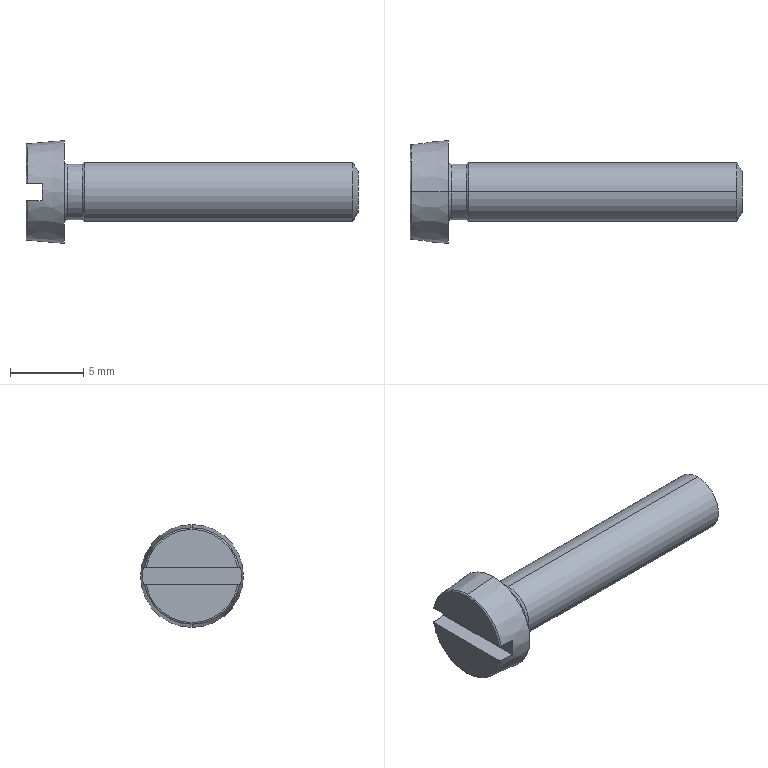Part | SolidWorks | features Cut 1, LPattern 1, RevCut 1, Revolution 1 | 1 solid | 22 faces | box 22.6 x 7 x 7 mm | volume 333.571 mm3 | plane 7 | cone 6 | torus 5 | cylinder 4 | commonest cylinder face diameters 3.8 x2 4 x2
STEP:
#1=CARTESIAN_POINT('',(22.6,0.,1.394));
#2=VERTEX_POINT('',#1);
#3=CARTESIAN_POINT('',(22.6,0.,-1.394));
#4=VERTEX_POINT('',#3);
#5=CARTESIAN_POINT('',(22.6,0.,0.));
#6=DIRECTION('',(-1.,0.,0.));
#7=DIRECTION('',(0.,0.,1.));
#8=AXIS2_PLACEMENT_3D('',#5,#6,#7);
#9=CIRCLE('',#8,1.394);
#10=EDGE_CURVE('',#2,#4,#9,.T.);
#11=ORIENTED_EDGE('',*,*,#10,.T.);
#12=CARTESIAN_POINT('',(22.25,0.,-2.));
#13=VERTEX_POINT('',#12);
#14=CARTESIAN_POINT('',(22.25,0.,-2.));
#15=DIRECTION('',(-0.5,0.,-0.866));
#16=VECTOR('',#15,1000.);
#17=LINE('',#14,#16);
#18=EDGE_CURVE('',#4,#13,#17,.T.);
#19=ORIENTED_EDGE('',*,*,#18,.T.);
#20=CARTESIAN_POINT('',(22.25,0.,2.));
#21=VERTEX_POINT('',#20);
#22=CARTESIAN_POINT('',(22.25,0.,0.));
#23=DIRECTION('',(-1.,0.,0.));
#24=DIRECTION('',(0.,0.,1.));
#25=AXIS2_PLACEMENT_3D('',#22,#23,#24);
#26=CIRCLE('',#25,2.);
#27=EDGE_CURVE('',#21,#13,#26,.T.);
#28=ORIENTED_EDGE('',*,*,#27,.F.);
#29=CARTESIAN_POINT('',(22.25,0.,2.));
#30=DIRECTION('',(-0.5,0.,0.866));
#31=VECTOR('',#30,1000.);
#32=LINE('',#29,#31);
#33=EDGE_CURVE('',#2,#21,#32,.T.);
#34=ORIENTED_EDGE('',*,*,#33,.F.);
#35=EDGE_LOOP('',(#11,#19,#28,#34));
#36=FACE_OUTER_BOUND('',#35,.T.);
#37=CARTESIAN_POINT('',(22.25,0.,0.));
#38=DIRECTION('',(-1.,0.,0.));
#39=DIRECTION('',(0.,0.,1.));
#40=AXIS2_PLACEMENT_3D('',#37,#38,#39);
#41=CONICAL_SURFACE('',#40,2.,1.047);
#42=ADVANCED_FACE('',(#36),#41,.T.);
#43=CARTESIAN_POINT('',(3.827,0.,1.9));
#44=VERTEX_POINT('',#43);
#45=CARTESIAN_POINT('',(3.827,0.,-1.9));
#46=VERTEX_POINT('',#45);
#47=CARTESIAN_POINT('',(3.827,0.,0.));
#48=DIRECTION('',(-1.,0.,0.));
#49=DIRECTION('',(0.,0.,1.));
#50=AXIS2_PLACEMENT_3D('',#47,#48,#49);
#51=CIRCLE('',#50,1.9);
#52=EDGE_CURVE('',#44,#46,#51,.T.);
#53=ORIENTED_EDGE('',*,*,#52,.F.);
#54=CARTESIAN_POINT('',(4.,0.,2.));
#55=VERTEX_POINT('',#54);
#56=CARTESIAN_POINT('',(4.,0.,2.));
#57=DIRECTION('',(0.866,0.,0.5));
#58=VECTOR('',#57,1000.);
#59=LINE('',#56,#58);
#60=EDGE_CURVE('',#44,#55,#59,.T.);
#61=ORIENTED_EDGE('',*,*,#60,.T.);
#62=CARTESIAN_POINT('',(4.,0.,-2.));
#63=VERTEX_POINT('',#62);
#64=CARTESIAN_POINT('',(4.,0.,0.));
#65=DIRECTION('',(-1.,0.,0.));
#66=DIRECTION('',(0.,0.,1.));
#67=AXIS2_PLACEMENT_3D('',#64,#65,#66);
#68=CIRCLE('',#67,2.);
#69=EDGE_CURVE('',#55,#63,#68,.T.);
#70=ORIENTED_EDGE('',*,*,#69,.T.);
#71=CARTESIAN_POINT('',(4.,0.,-2.));
#72=DIRECTION('',(0.866,0.,-0.5));
#73=VECTOR('',#72,1000.);
#74=LINE('',#71,#73);
#75=EDGE_CURVE('',#46,#63,#74,.T.);
#76=ORIENTED_EDGE('',*,*,#75,.F.);
#77=EDGE_LOOP('',(#53,#61,#70,#76));
#78=FACE_OUTER_BOUND('',#77,.T.);
#79=CARTESIAN_POINT('',(4.,0.,0.));
#80=DIRECTION('',(1.,0.,0.));
#81=DIRECTION('',(0.,0.,-1.));
#82=AXIS2_PLACEMENT_3D('',#79,#80,#81);
#83=CONICAL_SURFACE('',#82,2.,0.5236);
#84=ADVANCED_FACE('',(#78),#83,.T.);
#85=ORIENTED_EDGE('',*,*,#52,.T.);
#86=CARTESIAN_POINT('',(2.8,0.,-1.9));
#87=VERTEX_POINT('',#86);
#88=CARTESIAN_POINT('',(0.,0.,-1.9));
#89=DIRECTION('',(-1.,0.,0.));
#90=VECTOR('',#89,1000.);
#91=LINE('',#88,#90);
#92=EDGE_CURVE('',#46,#87,#91,.T.);
#93=ORIENTED_EDGE('',*,*,#92,.T.);
#94=CARTESIAN_POINT('',(2.8,0.,1.9));
#95=VERTEX_POINT('',#94);
#96=CARTESIAN_POINT('',(2.8,0.,0.));
#97=DIRECTION('',(-1.,0.,0.));
#98=DIRECTION('',(0.,0.,1.));
#99=AXIS2_PLACEMENT_3D('',#96,#97,#98);
#100=CIRCLE('',#99,1.9);
#101=EDGE_CURVE('',#95,#87,#100,.T.);
#102=ORIENTED_EDGE('',*,*,#101,.F.);
#103=CARTESIAN_POINT('',(0.,0.,1.9));
#104=DIRECTION('',(-1.,0.,0.));
#105=VECTOR('',#104,1000.);
#106=LINE('',#103,#105);
#107=EDGE_CURVE('',#44,#95,#106,.T.);
#108=ORIENTED_EDGE('',*,*,#107,.F.);
#109=EDGE_LOOP('',(#85,#93,#102,#108));
#110=FACE_OUTER_BOUND('',#109,.T.);
#111=CARTESIAN_POINT('',(0.,0.,0.));
#112=DIRECTION('',(-1.,0.,0.));
#113=DIRECTION('',(0.,0.,1.));
#114=AXIS2_PLACEMENT_3D('',#111,#112,#113);
#115=CYLINDRICAL_SURFACE('',#114,1.9);
#116=ADVANCED_FACE('',(#110),#115,.T.);
#117=CARTESIAN_POINT('',(2.6,0.,-2.1));
#118=VERTEX_POINT('',#117);
#119=CARTESIAN_POINT('',(2.6,0.,2.1));
#120=VERTEX_POINT('',#119);
#121=CARTESIAN_POINT('',(2.6,0.,0.));
#122=DIRECTION('',(-1.,0.,0.));
#123=DIRECTION('',(0.,0.,1.));
#124=AXIS2_PLACEMENT_3D('',#121,#122,#123);
#125=CIRCLE('',#124,2.1);
#126=EDGE_CURVE('',#118,#120,#125,.T.);
#127=ORIENTED_EDGE('',*,*,#126,.F.);
#128=CARTESIAN_POINT('',(2.8,0.,-2.1));
#129=DIRECTION('',(0.,1.,0.));
#130=DIRECTION('',(0.,0.,1.));
#131=AXIS2_PLACEMENT_3D('',#128,#129,#130);
#132=CIRCLE('',#131,0.2);
#133=EDGE_CURVE('',#118,#87,#132,.T.);
#134=ORIENTED_EDGE('',*,*,#133,.T.);
#135=CARTESIAN_POINT('',(2.8,0.,0.));
#136=DIRECTION('',(-1.,0.,0.));
#137=DIRECTION('',(0.,0.,1.));
#138=AXIS2_PLACEMENT_3D('',#135,#136,#137);
#139=CIRCLE('',#138,1.9);
#140=EDGE_CURVE('',#87,#95,#139,.T.);
#141=ORIENTED_EDGE('',*,*,#140,.T.);
#142=CARTESIAN_POINT('',(2.8,0.,2.1));
#143=DIRECTION('',(0.,-1.,0.));
#144=DIRECTION('',(0.,0.,-1.));
#145=AXIS2_PLACEMENT_3D('',#142,#143,#144);
#146=CIRCLE('',#145,0.2);
#147=EDGE_CURVE('',#120,#95,#146,.T.);
#148=ORIENTED_EDGE('',*,*,#147,.F.);
#149=EDGE_LOOP('',(#127,#134,#141,#148));
#150=FACE_OUTER_BOUND('',#149,.T.);
#151=CARTESIAN_POINT('',(2.8,0.,0.));
#152=DIRECTION('',(-1.,0.,0.));
#153=DIRECTION('',(0.,0.,1.));
#154=AXIS2_PLACEMENT_3D('',#151,#152,#153);
#155=TOROIDAL_SURFACE('',#154,2.1,0.2);
#156=ADVANCED_FACE('',(#150),#155,.F.);
#157=CARTESIAN_POINT('',(0.09128,0.,3.281));
#158=VERTEX_POINT('',#157);
#159=CARTESIAN_POINT('',(0.09128,3.225,0.6));
#160=VERTEX_POINT('',#159);
#161=CARTESIAN_POINT('',(0.09128,0.,0.));
#162=DIRECTION('',(-1.,0.,0.));
#163=DIRECTION('',(0.,0.,1.));
#164=AXIS2_PLACEMENT_3D('',#161,#162,#163);
#165=CIRCLE('',#164,3.281);
#166=EDGE_CURVE('',#158,#160,#165,.T.);
#167=ORIENTED_EDGE('',*,*,#166,.F.);
#168=CARTESIAN_POINT('',(2.6,0.,3.5));
#169=VERTEX_POINT('',#168);
#170=CARTESIAN_POINT('',(2.6,0.,3.5));
#171=DIRECTION('',(0.9962,0.,0.08716));
#172=VECTOR('',#171,1000.);
#173=LINE('',#170,#172);
#174=EDGE_CURVE('',#158,#169,#173,.T.);
#175=ORIENTED_EDGE('',*,*,#174,.T.);
#176=CARTESIAN_POINT('',(2.6,0.,-3.5));
#177=VERTEX_POINT('',#176);
#178=CARTESIAN_POINT('',(2.6,0.,0.));
#179=DIRECTION('',(-1.,0.,0.));
#180=DIRECTION('',(0.,0.,1.));
#181=AXIS2_PLACEMENT_3D('',#178,#179,#180);
#182=CIRCLE('',#181,3.5);
#183=EDGE_CURVE('',#169,#177,#182,.T.);
#184=ORIENTED_EDGE('',*,*,#183,.T.);
#185=CARTESIAN_POINT('',(0.09128,0.,-3.281));
#186=VERTEX_POINT('',#185);
#187=CARTESIAN_POINT('',(2.6,0.,-3.5));
#188=DIRECTION('',(0.9962,0.,-0.08716));
#189=VECTOR('',#188,1000.);
#190=LINE('',#187,#189);
#191=EDGE_CURVE('',#186,#177,#190,.T.);
#192=ORIENTED_EDGE('',*,*,#191,.F.);
#193=CARTESIAN_POINT('',(0.09128,3.225,-0.6));
#194=VERTEX_POINT('',#193);
#195=CARTESIAN_POINT('',(0.09128,0.,0.));
#196=DIRECTION('',(-1.,0.,0.));
#197=DIRECTION('',(0.,0.,1.));
#198=AXIS2_PLACEMENT_3D('',#195,#196,#197);
#199=CIRCLE('',#198,3.281);
#200=EDGE_CURVE('',#194,#186,#199,.T.);
#201=ORIENTED_EDGE('',*,*,#200,.F.);
#202=CARTESIAN_POINT('',(1.1,3.315,-0.6));
#203=VERTEX_POINT('',#202);
#204=CARTESIAN_POINT('',(0.09128,3.225,-0.6));
#205=CARTESIAN_POINT('',(0.2391,3.238,-0.6));
#206=CARTESIAN_POINT('',(0.3869,3.251,-0.6));
#207=CARTESIAN_POINT('',(0.5347,3.265,-0.6));
#208=CARTESIAN_POINT('',(0.7232,3.281,-0.6));
#209=CARTESIAN_POINT('',(0.9116,3.298,-0.6));
#210=CARTESIAN_POINT('',(1.1,3.315,-0.6));
#211=B_SPLINE_CURVE_WITH_KNOTS('',3,(#204,#205,#206,#207,#208,#209,#210),.UNSPECIFIED.,.F.,.F.,(4,3,4),(0.005661,0.006106,0.006674),.UNSPECIFIED.);
#212=EDGE_CURVE('',#194,#203,#211,.T.);
#213=ORIENTED_EDGE('',*,*,#212,.T.);
#214=CARTESIAN_POINT('',(1.1,3.315,0.6));
#215=VERTEX_POINT('',#214);
#216=CARTESIAN_POINT('',(1.1,0.,0.));
#217=DIRECTION('',(-1.,0.,0.));
#218=DIRECTION('',(0.,-1.,0.));
#219=AXIS2_PLACEMENT_3D('',#216,#217,#218);
#220=CIRCLE('',#219,3.369);
#221=EDGE_CURVE('',#215,#203,#220,.T.);
#222=ORIENTED_EDGE('',*,*,#221,.F.);
#223=CARTESIAN_POINT('',(1.1,3.315,0.6));
#224=CARTESIAN_POINT('',(0.9116,3.298,0.6));
#225=CARTESIAN_POINT('',(0.7232,3.281,0.6));
#226=CARTESIAN_POINT('',(0.5347,3.265,0.6));
#227=CARTESIAN_POINT('',(0.3869,3.251,0.6));
#228=CARTESIAN_POINT('',(0.2391,3.238,0.6));
#229=CARTESIAN_POINT('',(0.09128,3.225,0.6));
#230=B_SPLINE_CURVE_WITH_KNOTS('',3,(#223,#224,#225,#226,#227,#228,#229),.UNSPECIFIED.,.F.,.F.,(4,3,4),(0.005539,0.006106,0.006552),.UNSPECIFIED.);
#231=EDGE_CURVE('',#215,#160,#230,.T.);
#232=ORIENTED_EDGE('',*,*,#231,.T.);
#233=EDGE_LOOP('',(#167,#175,#184,#192,#201,#213,#222,#232));
#234=FACE_OUTER_BOUND('',#233,.T.);
#235=CARTESIAN_POINT('',(2.6,0.,0.));
#236=DIRECTION('',(1.,0.,0.));
#237=DIRECTION('',(0.,0.,-1.));
#238=AXIS2_PLACEMENT_3D('',#235,#236,#237);
#239=CONICAL_SURFACE('',#238,3.5,0.08727);
#240=ADVANCED_FACE('',(#234),#239,.T.);
#241=CARTESIAN_POINT('',(0.09128,-3.225,0.6));
#242=VERTEX_POINT('',#241);
#243=CARTESIAN_POINT('',(0.09128,0.,0.));
#244=DIRECTION('',(-1.,0.,0.));
#245=DIRECTION('',(0.,0.,1.));
#246=AXIS2_PLACEMENT_3D('',#243,#244,#245);
#247=CIRCLE('',#246,3.281);
#248=EDGE_CURVE('',#242,#158,#247,.T.);
#249=ORIENTED_EDGE('',*,*,#248,.T.);
#250=CARTESIAN_POINT('',(0.,0.,3.181));
#251=VERTEX_POINT('',#250);
#252=CARTESIAN_POINT('',(0.1,0.,3.181));
#253=DIRECTION('',(0.,-1.,0.));
#254=DIRECTION('',(0.,0.,-1.));
#255=AXIS2_PLACEMENT_3D('',#252,#253,#254);
#256=CIRCLE('',#255,0.1);
#257=EDGE_CURVE('',#158,#251,#256,.T.);
#258=ORIENTED_EDGE('',*,*,#257,.T.);
#259=CARTESIAN_POINT('',(0.,-3.124,0.6));
#260=VERTEX_POINT('',#259);
#261=CARTESIAN_POINT('',(0.,0.,0.));
#262=DIRECTION('',(-1.,0.,0.));
#263=DIRECTION('',(0.,0.,1.));
#264=AXIS2_PLACEMENT_3D('',#261,#262,#263);
#265=CIRCLE('',#264,3.181);
#266=EDGE_CURVE('',#260,#251,#265,.T.);
#267=ORIENTED_EDGE('',*,*,#266,.F.);
#268=CARTESIAN_POINT('',(0.,-3.124,0.6));
#269=CARTESIAN_POINT('',(0.,-3.127,0.6));
#270=CARTESIAN_POINT('',(0.0001152,-3.129,0.6));
#271=CARTESIAN_POINT('',(0.0003451,-3.132,0.6));
#272=CARTESIAN_POINT('',(0.001291,-3.144,0.6));
#273=CARTESIAN_POINT('',(0.004245,-3.155,0.6));
#274=CARTESIAN_POINT('',(0.008978,-3.166,0.6));
#275=CARTESIAN_POINT('',(0.01369,-3.177,0.6));
#276=CARTESIAN_POINT('',(0.02031,-3.186,0.6));
#277=CARTESIAN_POINT('',(0.0283,-3.195,0.6));
#278=CARTESIAN_POINT('',(0.03617,-3.203,0.6));
#279=CARTESIAN_POINT('',(0.0456,-3.21,0.6));
#280=CARTESIAN_POINT('',(0.05579,-3.215,0.6));
#281=CARTESIAN_POINT('',(0.06214,-3.218,0.6));
#282=CARTESIAN_POINT('',(0.06887,-3.221,0.6));
#283=CARTESIAN_POINT('',(0.07575,-3.223,0.6));
#284=CARTESIAN_POINT('',(0.08084,-3.224,0.6));
#285=CARTESIAN_POINT('',(0.08605,-3.225,0.6));
#286=CARTESIAN_POINT('',(0.09128,-3.225,0.6));
#287=B_SPLINE_CURVE_WITH_KNOTS('',3,(#268,#269,#270,#271,#272,#273,#274,#275,#276,#277,#278,#279,#280,#281,#282,#283,#284,#285,#286),.UNSPECIFIED.,.F.,.F.,(4,3,3,3,3,3,4),(0.0004978,0.0005062,0.000541,0.0005757,0.00061,0.0006311,0.0006468),.UNSPECIFIED.);
#288=EDGE_CURVE('',#260,#242,#287,.T.);
#289=ORIENTED_EDGE('',*,*,#288,.T.);
#290=EDGE_LOOP('',(#249,#258,#267,#289));
#291=FACE_OUTER_BOUND('',#290,.T.);
#292=CARTESIAN_POINT('',(0.1,0.,0.));
#293=DIRECTION('',(-1.,0.,0.));
#294=DIRECTION('',(0.,0.,1.));
#295=AXIS2_PLACEMENT_3D('',#292,#293,#294);
#296=TOROIDAL_SURFACE('',#295,3.181,0.1);
#297=ADVANCED_FACE('',(#291),#296,.T.);
#298=ORIENTED_EDGE('',*,*,#27,.T.);
#299=CARTESIAN_POINT('',(0.,0.,-2.));
#300=DIRECTION('',(-1.,0.,0.));
#301=VECTOR('',#300,1000.);
#302=LINE('',#299,#301);
#303=EDGE_CURVE('',#13,#63,#302,.T.);
#304=ORIENTED_EDGE('',*,*,#303,.T.);
#305=ORIENTED_EDGE('',*,*,#69,.F.);
#306=CARTESIAN_POINT('',(0.,0.,2.));
#307=DIRECTION('',(-1.,0.,0.));
#308=VECTOR('',#307,1000.);
#309=LINE('',#306,#308);
#310=EDGE_CURVE('',#21,#55,#309,.T.);
#311=ORIENTED_EDGE('',*,*,#310,.F.);
#312=EDGE_LOOP('',(#298,#304,#305,#311));
#313=FACE_OUTER_BOUND('',#312,.T.);
#314=CARTESIAN_POINT('',(0.,0.,0.));
#315=DIRECTION('',(-1.,0.,0.));
#316=DIRECTION('',(0.,0.,1.));
#317=AXIS2_PLACEMENT_3D('',#314,#315,#316);
#318=CYLINDRICAL_SURFACE('',#317,2.);
#319=ADVANCED_FACE('',(#313),#318,.T.);
#320=ORIENTED_EDGE('',*,*,#303,.F.);
#321=CARTESIAN_POINT('',(22.25,0.,0.));
#322=DIRECTION('',(-1.,0.,0.));
#323=DIRECTION('',(0.,0.,1.));
#324=AXIS2_PLACEMENT_3D('',#321,#322,#323);
#325=CIRCLE('',#324,2.);
#326=EDGE_CURVE('',#13,#21,#325,.T.);
#327=ORIENTED_EDGE('',*,*,#326,.T.);
#328=ORIENTED_EDGE('',*,*,#310,.T.);
#329=CARTESIAN_POINT('',(4.,0.,0.));
#330=DIRECTION('',(-1.,0.,0.));
#331=DIRECTION('',(0.,0.,1.));
#332=AXIS2_PLACEMENT_3D('',#329,#330,#331);
#333=CIRCLE('',#332,2.);
#334=EDGE_CURVE('',#63,#55,#333,.T.);
#335=ORIENTED_EDGE('',*,*,#334,.F.);
#336=EDGE_LOOP('',(#320,#327,#328,#335));
#337=FACE_OUTER_BOUND('',#336,.T.);
#338=CARTESIAN_POINT('',(0.,0.,0.));
#339=DIRECTION('',(-1.,0.,0.));
#340=DIRECTION('',(0.,0.,1.));
#341=AXIS2_PLACEMENT_3D('',#338,#339,#340);
#342=CYLINDRICAL_SURFACE('',#341,2.);
#343=ADVANCED_FACE('',(#337),#342,.T.);
#344=ORIENTED_EDGE('',*,*,#266,.T.);
#345=CARTESIAN_POINT('',(0.,3.124,0.6));
#346=VERTEX_POINT('',#345);
#347=CARTESIAN_POINT('',(0.,0.,0.));
#348=DIRECTION('',(-1.,0.,0.));
#349=DIRECTION('',(0.,0.,1.));
#350=AXIS2_PLACEMENT_3D('',#347,#348,#349);
#351=CIRCLE('',#350,3.181);
#352=EDGE_CURVE('',#251,#346,#351,.T.);
#353=ORIENTED_EDGE('',*,*,#352,.T.);
#354=CARTESIAN_POINT('',(0.,3.448,0.6));
#355=DIRECTION('',(0.,1.,0.));
#356=VECTOR('',#355,1000.);
#357=LINE('',#354,#356);
#358=EDGE_CURVE('',#260,#346,#357,.T.);
#359=ORIENTED_EDGE('',*,*,#358,.F.);
#360=EDGE_LOOP('',(#344,#353,#359));
#361=FACE_OUTER_BOUND('',#360,.T.);
#362=CARTESIAN_POINT('',(0.,0.,0.));
#363=DIRECTION('',(1.,0.,0.));
#364=DIRECTION('',(0.,0.,-1.));
#365=AXIS2_PLACEMENT_3D('',#362,#363,#364);
#366=PLANE('',#365);
#367=ADVANCED_FACE('',(#361),#366,.F.);
#368=ORIENTED_EDGE('',*,*,#257,.F.);
#369=ORIENTED_EDGE('',*,*,#166,.T.);
#370=CARTESIAN_POINT('',(0.09128,3.225,0.6));
#371=CARTESIAN_POINT('',(0.08575,3.225,0.6));
#372=CARTESIAN_POINT('',(0.08024,3.224,0.6));
#373=CARTESIAN_POINT('',(0.07487,3.222,0.6));
#374=CARTESIAN_POINT('',(0.06423,3.219,0.6));
#375=CARTESIAN_POINT('',(0.05392,3.215,0.6));
#376=CARTESIAN_POINT('',(0.04479,3.209,0.6));
#377=CARTESIAN_POINT('',(0.03559,3.202,0.6));
#378=CARTESIAN_POINT('',(0.02733,3.195,0.6));
#379=CARTESIAN_POINT('',(0.02065,3.186,0.6));
#380=CARTESIAN_POINT('',(0.01387,3.177,0.6));
#381=CARTESIAN_POINT('',(0.008539,3.166,0.6));
#382=CARTESIAN_POINT('',(0.005059,3.156,0.6));
#383=CARTESIAN_POINT('',(0.001724,3.146,0.6));
#384=CARTESIAN_POINT('',(0.,3.135,0.6));
#385=CARTESIAN_POINT('',(0.,3.124,0.6));
#386=B_SPLINE_CURVE_WITH_KNOTS('',3,(#370,#371,#372,#373,#374,#375,#376,#377,#378,#379,#380,#381,#382,#383,#384,#385),.UNSPECIFIED.,.F.,.F.,(4,3,3,3,3,4),(0.0003882,0.0004048,0.0004379,0.0004711,0.0005049,0.0005373),.UNSPECIFIED.);
#387=EDGE_CURVE('',#160,#346,#386,.T.);
#388=ORIENTED_EDGE('',*,*,#387,.T.);
#389=ORIENTED_EDGE('',*,*,#352,.F.);
#390=EDGE_LOOP('',(#368,#369,#388,#389));
#391=FACE_OUTER_BOUND('',#390,.T.);
#392=CARTESIAN_POINT('',(0.1,0.,0.));
#393=DIRECTION('',(-1.,0.,0.));
#394=DIRECTION('',(0.,0.,1.));
#395=AXIS2_PLACEMENT_3D('',#392,#393,#394);
#396=TOROIDAL_SURFACE('',#395,3.181,0.1);
#397=ADVANCED_FACE('',(#391),#396,.T.);
#398=CARTESIAN_POINT('',(0.,3.124,-0.6));
#399=VERTEX_POINT('',#398);
#400=CARTESIAN_POINT('',(0.,-3.124,-0.6));
#401=VERTEX_POINT('',#400);
#402=CARTESIAN_POINT('',(0.,0.,0.));
#403=DIRECTION('',(-1.,0.,0.));
#404=DIRECTION('',(0.,0.,1.));
#405=AXIS2_PLACEMENT_3D('',#402,#403,#404);
#406=CIRCLE('',#405,3.181);
#407=EDGE_CURVE('',#399,#401,#406,.T.);
#408=ORIENTED_EDGE('',*,*,#407,.T.);
#409=CARTESIAN_POINT('',(0.,3.448,-0.6));
#410=DIRECTION('',(0.,-1.,0.));
#411=VECTOR('',#410,1000.);
#412=LINE('',#409,#411);
#413=EDGE_CURVE('',#399,#401,#412,.T.);
#414=ORIENTED_EDGE('',*,*,#413,.F.);
#415=EDGE_LOOP('',(#408,#414));
#416=FACE_OUTER_BOUND('',#415,.T.);
#417=CARTESIAN_POINT('',(0.,0.,0.));
#418=DIRECTION('',(1.,0.,0.));
#419=DIRECTION('',(0.,0.,-1.));
#420=AXIS2_PLACEMENT_3D('',#417,#418,#419);
#421=PLANE('',#420);
#422=ADVANCED_FACE('',(#416),#421,.F.);
#423=ORIENTED_EDGE('',*,*,#200,.T.);
#424=CARTESIAN_POINT('',(0.09128,-3.225,-0.6));
#425=VERTEX_POINT('',#424);
#426=CARTESIAN_POINT('',(0.09128,0.,0.));
#427=DIRECTION('',(-1.,0.,0.));
#428=DIRECTION('',(0.,0.,1.));
#429=AXIS2_PLACEMENT_3D('',#426,#427,#428);
#430=CIRCLE('',#429,3.281);
#431=EDGE_CURVE('',#186,#425,#430,.T.);
#432=ORIENTED_EDGE('',*,*,#431,.T.);
#433=CARTESIAN_POINT('',(0.09128,-3.225,-0.6));
#434=CARTESIAN_POINT('',(0.08605,-3.225,-0.6));
#435=CARTESIAN_POINT('',(0.08084,-3.224,-0.6));
#436=CARTESIAN_POINT('',(0.07575,-3.223,-0.6));
#437=CARTESIAN_POINT('',(0.06495,-3.22,-0.6));
#438=CARTESIAN_POINT('',(0.05448,-3.215,-0.6));
#439=CARTESIAN_POINT('',(0.04521,-3.209,-0.6));
#440=CARTESIAN_POINT('',(0.03594,-3.203,-0.6));
#441=CARTESIAN_POINT('',(0.02761,-3.195,-0.6));
#442=CARTESIAN_POINT('',(0.02088,-3.186,-0.6));
#443=CARTESIAN_POINT('',(0.01407,-3.177,-0.6));
#444=CARTESIAN_POINT('',(0.008699,-3.167,-0.6));
#445=CARTESIAN_POINT('',(0.005179,-3.156,-0.6));
#446=CARTESIAN_POINT('',(0.001766,-3.146,-0.6));
#447=CARTESIAN_POINT('',(0.,-3.135,-0.6));
#448=CARTESIAN_POINT('',(0.,-3.124,-0.6));
#449=B_SPLINE_CURVE_WITH_KNOTS('',3,(#433,#434,#435,#436,#437,#438,#439,#440,#441,#442,#443,#444,#445,#446,#447,#448),.UNSPECIFIED.,.F.,.F.,(4,3,3,3,3,4),(0.0006154,0.000631,0.0006644,0.0006978,0.0007316,0.0007643),.UNSPECIFIED.);
#450=EDGE_CURVE('',#425,#401,#449,.T.);
#451=ORIENTED_EDGE('',*,*,#450,.T.);
#452=ORIENTED_EDGE('',*,*,#407,.F.);
#453=CARTESIAN_POINT('',(0.,3.124,-0.6));
#454=CARTESIAN_POINT('',(0.,3.127,-0.6));
#455=CARTESIAN_POINT('',(0.0001277,3.13,-0.6));
#456=CARTESIAN_POINT('',(0.0003824,3.133,-0.6));
#457=CARTESIAN_POINT('',(0.001378,3.144,-0.6));
#458=CARTESIAN_POINT('',(0.004382,3.156,-0.6));
#459=CARTESIAN_POINT('',(0.009162,3.166,-0.6));
#460=CARTESIAN_POINT('',(0.01392,3.177,-0.6));
#461=CARTESIAN_POINT('',(0.02058,3.187,-0.6));
#462=CARTESIAN_POINT('',(0.0286,3.195,-0.6));
#463=CARTESIAN_POINT('',(0.03651,3.203,-0.6));
#464=CARTESIAN_POINT('',(0.04597,3.21,-0.6));
#465=CARTESIAN_POINT('',(0.05618,3.215,-0.6));
#466=CARTESIAN_POINT('',(0.06622,3.22,-0.6));
#467=CARTESIAN_POINT('',(0.07726,3.224,-0.6));
#468=CARTESIAN_POINT('',(0.08839,3.225,-0.6));
#469=CARTESIAN_POINT('',(0.08935,3.225,-0.6));
#470=CARTESIAN_POINT('',(0.09032,3.225,-0.6));
#471=CARTESIAN_POINT('',(0.09128,3.225,-0.6));
#472=B_SPLINE_CURVE_WITH_KNOTS('',3,(#453,#454,#455,#456,#457,#458,#459,#460,#461,#462,#463,#464,#465,#466,#467,#468,#469,#470,#471),.UNSPECIFIED.,.F.,.F.,(4,3,3,3,3,3,4),(0.00009389,0.0001027,0.0001375,0.0001722,0.0002064,0.00024,0.0002429),.UNSPECIFIED.);
#473=EDGE_CURVE('',#399,#194,#472,.T.);
#474=ORIENTED_EDGE('',*,*,#473,.T.);
#475=EDGE_LOOP('',(#423,#432,#451,#452,#474));
#476=FACE_OUTER_BOUND('',#475,.T.);
#477=CARTESIAN_POINT('',(0.1,0.,0.));
#478=DIRECTION('',(-1.,0.,0.));
#479=DIRECTION('',(0.,0.,1.));
#480=AXIS2_PLACEMENT_3D('',#477,#478,#479);
#481=TOROIDAL_SURFACE('',#480,3.181,0.1);
#482=ADVANCED_FACE('',(#476),#481,.T.);
#483=ORIENTED_EDGE('',*,*,#174,.F.);
#484=ORIENTED_EDGE('',*,*,#248,.F.);
#485=CARTESIAN_POINT('',(1.1,-3.315,0.6));
#486=VERTEX_POINT('',#485);
#487=CARTESIAN_POINT('',(0.09128,-3.225,0.6));
#488=CARTESIAN_POINT('',(0.2391,-3.238,0.6));
#489=CARTESIAN_POINT('',(0.3869,-3.251,0.6));
#490=CARTESIAN_POINT('',(0.5347,-3.265,0.6));
#491=CARTESIAN_POINT('',(0.7232,-3.281,0.6));
#492=CARTESIAN_POINT('',(0.9116,-3.298,0.6));
#493=CARTESIAN_POINT('',(1.1,-3.315,0.6));
#494=B_SPLINE_CURVE_WITH_KNOTS('',3,(#487,#488,#489,#490,#491,#492,#493),.UNSPECIFIED.,.F.,.F.,(4,3,4),(0.005661,0.006106,0.006674),.UNSPECIFIED.);
#495=EDGE_CURVE('',#242,#486,#494,.T.);
#496=ORIENTED_EDGE('',*,*,#495,.T.);
#497=CARTESIAN_POINT('',(1.1,-3.315,-0.6));
#498=VERTEX_POINT('',#497);
#499=CARTESIAN_POINT('',(1.1,0.,0.));
#500=DIRECTION('',(-1.,0.,0.));
#501=DIRECTION('',(0.,-1.,0.));
#502=AXIS2_PLACEMENT_3D('',#499,#500,#501);
#503=CIRCLE('',#502,3.369);
#504=EDGE_CURVE('',#498,#486,#503,.T.);
#505=ORIENTED_EDGE('',*,*,#504,.F.);
#506=CARTESIAN_POINT('',(1.1,-3.315,-0.6));
#507=CARTESIAN_POINT('',(0.9116,-3.298,-0.6));
#508=CARTESIAN_POINT('',(0.7232,-3.281,-0.6));
#509=CARTESIAN_POINT('',(0.5347,-3.265,-0.6));
#510=CARTESIAN_POINT('',(0.3869,-3.251,-0.6));
#511=CARTESIAN_POINT('',(0.2391,-3.238,-0.6));
#512=CARTESIAN_POINT('',(0.09128,-3.225,-0.6));
#513=B_SPLINE_CURVE_WITH_KNOTS('',3,(#506,#507,#508,#509,#510,#511,#512),.UNSPECIFIED.,.F.,.F.,(4,3,4),(0.005539,0.006106,0.006552),.UNSPECIFIED.);
#514=EDGE_CURVE('',#498,#425,#513,.T.);
#515=ORIENTED_EDGE('',*,*,#514,.T.);
#516=ORIENTED_EDGE('',*,*,#431,.F.);
#517=ORIENTED_EDGE('',*,*,#191,.T.);
#518=CARTESIAN_POINT('',(2.6,0.,0.));
#519=DIRECTION('',(-1.,0.,0.));
#520=DIRECTION('',(0.,0.,1.));
#521=AXIS2_PLACEMENT_3D('',#518,#519,#520);
#522=CIRCLE('',#521,3.5);
#523=EDGE_CURVE('',#177,#169,#522,.T.);
#524=ORIENTED_EDGE('',*,*,#523,.T.);
#525=EDGE_LOOP('',(#483,#484,#496,#505,#515,#516,#517,#524));
#526=FACE_OUTER_BOUND('',#525,.T.);
#527=CARTESIAN_POINT('',(2.6,0.,0.));
#528=DIRECTION('',(1.,0.,0.));
#529=DIRECTION('',(0.,0.,-1.));
#530=AXIS2_PLACEMENT_3D('',#527,#528,#529);
#531=CONICAL_SURFACE('',#530,3.5,0.08727);
#532=ADVANCED_FACE('',(#526),#531,.T.);
#533=ORIENTED_EDGE('',*,*,#523,.F.);
#534=ORIENTED_EDGE('',*,*,#183,.F.);
#535=EDGE_LOOP('',(#533,#534));
#536=FACE_OUTER_BOUND('',#535,.T.);
#537=CARTESIAN_POINT('',(2.6,0.,0.));
#538=DIRECTION('',(-1.,0.,0.));
#539=DIRECTION('',(0.,0.,1.));
#540=AXIS2_PLACEMENT_3D('',#537,#538,#539);
#541=CIRCLE('',#540,2.1);
#542=EDGE_CURVE('',#120,#118,#541,.T.);
#543=ORIENTED_EDGE('',*,*,#542,.T.);
#544=ORIENTED_EDGE('',*,*,#126,.T.);
#545=EDGE_LOOP('',(#543,#544));
#546=FACE_BOUND('',#545,.T.);
#547=CARTESIAN_POINT('',(2.6,3.5,0.));
#548=DIRECTION('',(-1.,0.,0.));
#549=DIRECTION('',(0.,0.,1.));
#550=AXIS2_PLACEMENT_3D('',#547,#548,#549);
#551=PLANE('',#550);
#552=ADVANCED_FACE('',(#536,#546),#551,.F.);
#553=ORIENTED_EDGE('',*,*,#133,.F.);
#554=ORIENTED_EDGE('',*,*,#542,.F.);
#555=ORIENTED_EDGE('',*,*,#147,.T.);
#556=ORIENTED_EDGE('',*,*,#101,.T.);
#557=EDGE_LOOP('',(#553,#554,#555,#556));
#558=FACE_OUTER_BOUND('',#557,.T.);
#559=CARTESIAN_POINT('',(2.8,0.,0.));
#560=DIRECTION('',(-1.,0.,0.));
#561=DIRECTION('',(0.,0.,1.));
#562=AXIS2_PLACEMENT_3D('',#559,#560,#561);
#563=TOROIDAL_SURFACE('',#562,2.1,0.2);
#564=ADVANCED_FACE('',(#558),#563,.F.);
#565=ORIENTED_EDGE('',*,*,#92,.F.);
#566=CARTESIAN_POINT('',(3.827,0.,0.));
#567=DIRECTION('',(-1.,0.,0.));
#568=DIRECTION('',(0.,0.,1.));
#569=AXIS2_PLACEMENT_3D('',#566,#567,#568);
#570=CIRCLE('',#569,1.9);
#571=EDGE_CURVE('',#46,#44,#570,.T.);
#572=ORIENTED_EDGE('',*,*,#571,.T.);
#573=ORIENTED_EDGE('',*,*,#107,.T.);
#574=ORIENTED_EDGE('',*,*,#140,.F.);
#575=EDGE_LOOP('',(#565,#572,#573,#574));
#576=FACE_OUTER_BOUND('',#575,.T.);
#577=CARTESIAN_POINT('',(0.,0.,0.));
#578=DIRECTION('',(-1.,0.,0.));
#579=DIRECTION('',(0.,0.,1.));
#580=AXIS2_PLACEMENT_3D('',#577,#578,#579);
#581=CYLINDRICAL_SURFACE('',#580,1.9);
#582=ADVANCED_FACE('',(#576),#581,.T.);
#583=ORIENTED_EDGE('',*,*,#60,.F.);
#584=ORIENTED_EDGE('',*,*,#571,.F.);
#585=ORIENTED_EDGE('',*,*,#75,.T.);
#586=ORIENTED_EDGE('',*,*,#334,.T.);
#587=EDGE_LOOP('',(#583,#584,#585,#586));
#588=FACE_OUTER_BOUND('',#587,.T.);
#589=CARTESIAN_POINT('',(4.,0.,0.));
#590=DIRECTION('',(1.,0.,0.));
#591=DIRECTION('',(0.,0.,-1.));
#592=AXIS2_PLACEMENT_3D('',#589,#590,#591);
#593=CONICAL_SURFACE('',#592,2.,0.5236);
#594=ADVANCED_FACE('',(#588),#593,.T.);
#595=ORIENTED_EDGE('',*,*,#358,.T.);
#596=ORIENTED_EDGE('',*,*,#387,.F.);
#597=ORIENTED_EDGE('',*,*,#231,.F.);
#598=CARTESIAN_POINT('',(1.1,3.448,0.6));
#599=DIRECTION('',(0.,1.,0.));
#600=VECTOR('',#599,1000.);
#601=LINE('',#598,#600);
#602=EDGE_CURVE('',#486,#215,#601,.T.);
#603=ORIENTED_EDGE('',*,*,#602,.F.);
#604=ORIENTED_EDGE('',*,*,#495,.F.);
#605=ORIENTED_EDGE('',*,*,#288,.F.);
#606=EDGE_LOOP('',(#595,#596,#597,#603,#604,#605));
#607=FACE_OUTER_BOUND('',#606,.T.);
#608=CARTESIAN_POINT('',(1.1,3.448,0.6));
#609=DIRECTION('',(0.,0.,1.));
#610=DIRECTION('',(0.,-1.,0.));
#611=AXIS2_PLACEMENT_3D('',#608,#609,#610);
#612=PLANE('',#611);
#613=ADVANCED_FACE('',(#607),#612,.F.);
#614=ORIENTED_EDGE('',*,*,#514,.F.);
#615=CARTESIAN_POINT('',(1.1,3.448,-0.6));
#616=DIRECTION('',(0.,-1.,0.));
#617=VECTOR('',#616,1000.);
#618=LINE('',#615,#617);
#619=EDGE_CURVE('',#203,#498,#618,.T.);
#620=ORIENTED_EDGE('',*,*,#619,.F.);
#621=ORIENTED_EDGE('',*,*,#212,.F.);
#622=ORIENTED_EDGE('',*,*,#473,.F.);
#623=ORIENTED_EDGE('',*,*,#413,.T.);
#624=ORIENTED_EDGE('',*,*,#450,.F.);
#625=EDGE_LOOP('',(#614,#620,#621,#622,#623,#624));
#626=FACE_OUTER_BOUND('',#625,.T.);
#627=CARTESIAN_POINT('',(1.1,3.448,-0.6));
#628=DIRECTION('',(0.,0.,-1.));
#629=DIRECTION('',(-1.,0.,0.));
#630=AXIS2_PLACEMENT_3D('',#627,#628,#629);
#631=PLANE('',#630);
#632=ADVANCED_FACE('',(#626),#631,.F.);
#633=ORIENTED_EDGE('',*,*,#221,.T.);
#634=ORIENTED_EDGE('',*,*,#619,.T.);
#635=ORIENTED_EDGE('',*,*,#504,.T.);
#636=ORIENTED_EDGE('',*,*,#602,.T.);
#637=EDGE_LOOP('',(#633,#634,#635,#636));
#638=FACE_OUTER_BOUND('',#637,.T.);
#639=CARTESIAN_POINT('',(1.1,0.,0.));
#640=DIRECTION('',(-1.,0.,0.));
#641=DIRECTION('',(0.,-1.,0.));
#642=AXIS2_PLACEMENT_3D('',#639,#640,#641);
#643=PLANE('',#642);
#644=ADVANCED_FACE('',(#638),#643,.T.);
#645=ORIENTED_EDGE('',*,*,#18,.F.);
#646=CARTESIAN_POINT('',(22.6,0.,0.));
#647=DIRECTION('',(-1.,0.,0.));
#648=DIRECTION('',(0.,0.,1.));
#649=AXIS2_PLACEMENT_3D('',#646,#647,#648);
#650=CIRCLE('',#649,1.394);
#651=EDGE_CURVE('',#4,#2,#650,.T.);
#652=ORIENTED_EDGE('',*,*,#651,.T.);
#653=ORIENTED_EDGE('',*,*,#33,.T.);
#654=ORIENTED_EDGE('',*,*,#326,.F.);
#655=EDGE_LOOP('',(#645,#652,#653,#654));
#656=FACE_OUTER_BOUND('',#655,.T.);
#657=CARTESIAN_POINT('',(22.25,0.,0.));
#658=DIRECTION('',(-1.,0.,0.));
#659=DIRECTION('',(0.,0.,1.));
#660=AXIS2_PLACEMENT_3D('',#657,#658,#659);
#661=CONICAL_SURFACE('',#660,2.,1.047);
#662=ADVANCED_FACE('',(#656),#661,.T.);
#663=ORIENTED_EDGE('',*,*,#10,.F.);
#664=ORIENTED_EDGE('',*,*,#651,.F.);
#665=EDGE_LOOP('',(#663,#664));
#666=FACE_OUTER_BOUND('',#665,.T.);
#667=CARTESIAN_POINT('',(22.6,2.,0.));
#668=DIRECTION('',(-1.,0.,0.));
#669=DIRECTION('',(0.,0.,1.));
#670=AXIS2_PLACEMENT_3D('',#667,#668,#669);
#671=PLANE('',#670);
#672=ADVANCED_FACE('',(#666),#671,.F.);
#673=CLOSED_SHELL('',(#42,#84,#116,#156,#240,#297,#319,#343,#367,#397,#422,#482,#532,#552,#564,#582,#594,#613,#632,#644,#662,#672));
#674=MANIFOLD_SOLID_BREP('',#673);
#675=CARTESIAN_POINT('',(0.,0.,0.));
#676=DIRECTION('',(0.,0.,1.));
#677=DIRECTION('',(1.,0.,0.));
#678=AXIS2_PLACEMENT_3D('',#675,#676,#677);
#679=(LENGTH_UNIT()NAMED_UNIT(*)SI_UNIT(.MILLI.,.METRE.));
#680=UNCERTAINTY_MEASURE_WITH_UNIT(LENGTH_MEASURE(0.00001),#679,'','');
#681=(NAMED_UNIT(*)PLANE_ANGLE_UNIT()SI_UNIT($,.RADIAN.));
#682=(NAMED_UNIT(*)SI_UNIT($,.STERADIAN.)SOLID_ANGLE_UNIT());
#683=(GEOMETRIC_REPRESENTATION_CONTEXT(3)GLOBAL_UNCERTAINTY_ASSIGNED_CONTEXT((#680))GLOBAL_UNIT_ASSIGNED_CONTEXT((#679,#681,#682))REPRESENTATION_CONTEXT('',''));
#684=ADVANCED_BREP_SHAPE_REPRESENTATION('',(#674,#678),#683);